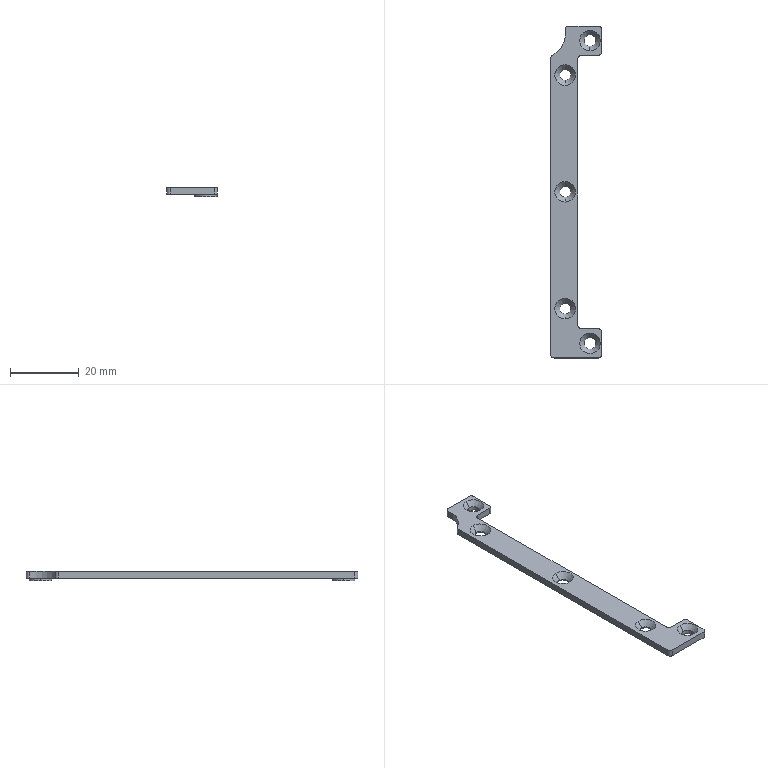Part | 1 solid | 46 faces | box 14.723 x 96.5 x 2.7 mm | volume 1577 mm3 | cylinder 24 | plane 12 | cone 10 | commonest cylinder face diameters 3.2 x6 2 x5 1.6 x4 3.4 x4 6.6 x4 14.8 x1
STEP:
#1=CARTESIAN_POINT('',(7.361,44.,-2.));
#2=VERTEX_POINT('',#1);
#3=CARTESIAN_POINT('',(0.7613,44.,-2.));
#4=VERTEX_POINT('',#3);
#5=CARTESIAN_POINT('',(4.061,44.,-2.));
#6=DIRECTION('',(0.,0.,-1.));
#7=DIRECTION('',(1.,0.,0.));
#8=AXIS2_PLACEMENT_3D('',#5,#6,#7);
#9=CIRCLE('',#8,3.3);
#10=EDGE_CURVE('',#2,#4,#9,.T.);
#11=ORIENTED_EDGE('',*,*,#10,.F.);
#12=CARTESIAN_POINT('',(7.361,40.55,-2.));
#13=VERTEX_POINT('',#12);
#14=CARTESIAN_POINT('',(7.361,40.55,-2.));
#15=DIRECTION('',(0.,1.,0.));
#16=VECTOR('',#15,1000.);
#17=LINE('',#14,#16);
#18=EDGE_CURVE('',#13,#2,#17,.T.);
#19=ORIENTED_EDGE('',*,*,#18,.F.);
#20=CARTESIAN_POINT('',(6.561,39.75,-2.));
#21=VERTEX_POINT('',#20);
#22=CARTESIAN_POINT('',(6.561,40.55,-2.));
#23=DIRECTION('',(0.,0.,1.));
#24=DIRECTION('',(0.,-1.,0.));
#25=AXIS2_PLACEMENT_3D('',#22,#23,#24);
#26=CIRCLE('',#25,0.8);
#27=EDGE_CURVE('',#21,#13,#26,.T.);
#28=ORIENTED_EDGE('',*,*,#27,.F.);
#29=CARTESIAN_POINT('',(1.561,39.75,-2.));
#30=VERTEX_POINT('',#29);
#31=CARTESIAN_POINT('',(1.561,39.75,-2.));
#32=DIRECTION('',(1.,0.,0.));
#33=VECTOR('',#32,1000.);
#34=LINE('',#31,#33);
#35=EDGE_CURVE('',#30,#21,#34,.T.);
#36=ORIENTED_EDGE('',*,*,#35,.F.);
#37=CARTESIAN_POINT('',(0.5613,38.75,-2.));
#38=VERTEX_POINT('',#37);
#39=CARTESIAN_POINT('',(1.561,38.75,-2.));
#40=DIRECTION('',(0.,0.,1.));
#41=DIRECTION('',(0.,1.,0.));
#42=AXIS2_PLACEMENT_3D('',#39,#40,#41);
#43=CIRCLE('',#42,1.);
#44=EDGE_CURVE('',#30,#38,#43,.T.);
#45=ORIENTED_EDGE('',*,*,#44,.T.);
#46=CARTESIAN_POINT('',(0.5613,-38.75,-2.));
#47=VERTEX_POINT('',#46);
#48=CARTESIAN_POINT('',(0.5613,-38.75,-2.));
#49=DIRECTION('',(0.,1.,0.));
#50=VECTOR('',#49,1000.);
#51=LINE('',#48,#50);
#52=EDGE_CURVE('',#47,#38,#51,.T.);
#53=ORIENTED_EDGE('',*,*,#52,.F.);
#54=CARTESIAN_POINT('',(1.561,-39.75,-2.));
#55=VERTEX_POINT('',#54);
#56=CARTESIAN_POINT('',(1.561,-38.75,-2.));
#57=DIRECTION('',(0.,0.,1.));
#58=DIRECTION('',(-1.,0.,0.));
#59=AXIS2_PLACEMENT_3D('',#56,#57,#58);
#60=CIRCLE('',#59,1.);
#61=EDGE_CURVE('',#47,#55,#60,.T.);
#62=ORIENTED_EDGE('',*,*,#61,.T.);
#63=CARTESIAN_POINT('',(6.561,-39.75,-2.));
#64=VERTEX_POINT('',#63);
#65=CARTESIAN_POINT('',(6.561,-39.75,-2.));
#66=DIRECTION('',(-1.,0.,0.));
#67=VECTOR('',#66,1000.);
#68=LINE('',#65,#67);
#69=EDGE_CURVE('',#64,#55,#68,.T.);
#70=ORIENTED_EDGE('',*,*,#69,.F.);
#71=CARTESIAN_POINT('',(7.361,-40.55,-2.));
#72=VERTEX_POINT('',#71);
#73=CARTESIAN_POINT('',(6.561,-40.55,-2.));
#74=DIRECTION('',(0.,0.,1.));
#75=DIRECTION('',(1.,0.,0.));
#76=AXIS2_PLACEMENT_3D('',#73,#74,#75);
#77=CIRCLE('',#76,0.8);
#78=EDGE_CURVE('',#72,#64,#77,.T.);
#79=ORIENTED_EDGE('',*,*,#78,.F.);
#80=CARTESIAN_POINT('',(7.361,-44.,-2.));
#81=VERTEX_POINT('',#80);
#82=CARTESIAN_POINT('',(7.361,-44.,-2.));
#83=DIRECTION('',(0.,1.,0.));
#84=VECTOR('',#83,1000.);
#85=LINE('',#82,#84);
#86=EDGE_CURVE('',#81,#72,#85,.T.);
#87=ORIENTED_EDGE('',*,*,#86,.F.);
#88=CARTESIAN_POINT('',(0.7613,-44.,-2.));
#89=VERTEX_POINT('',#88);
#90=CARTESIAN_POINT('',(4.061,-44.,-2.));
#91=DIRECTION('',(0.,0.,-1.));
#92=DIRECTION('',(-1.,0.,0.));
#93=AXIS2_PLACEMENT_3D('',#90,#91,#92);
#94=CIRCLE('',#93,3.3);
#95=EDGE_CURVE('',#89,#81,#94,.T.);
#96=ORIENTED_EDGE('',*,*,#95,.F.);
#97=CARTESIAN_POINT('',(4.061,-44.,-2.));
#98=DIRECTION('',(0.,0.,-1.));
#99=DIRECTION('',(1.,0.,0.));
#100=AXIS2_PLACEMENT_3D('',#97,#98,#99);
#101=CIRCLE('',#100,3.3);
#102=EDGE_CURVE('',#81,#89,#101,.T.);
#103=ORIENTED_EDGE('',*,*,#102,.F.);
#104=CARTESIAN_POINT('',(7.361,-47.45,-2.));
#105=VERTEX_POINT('',#104);
#106=CARTESIAN_POINT('',(7.361,-47.45,-2.));
#107=DIRECTION('',(0.,1.,0.));
#108=VECTOR('',#107,1000.);
#109=LINE('',#106,#108);
#110=EDGE_CURVE('',#105,#81,#109,.T.);
#111=ORIENTED_EDGE('',*,*,#110,.F.);
#112=CARTESIAN_POINT('',(6.561,-48.25,-2.));
#113=VERTEX_POINT('',#112);
#114=CARTESIAN_POINT('',(6.561,-47.45,-2.));
#115=DIRECTION('',(0.,0.,1.));
#116=DIRECTION('',(0.,-1.,0.));
#117=AXIS2_PLACEMENT_3D('',#114,#115,#116);
#118=CIRCLE('',#117,0.8);
#119=EDGE_CURVE('',#113,#105,#118,.T.);
#120=ORIENTED_EDGE('',*,*,#119,.F.);
#121=CARTESIAN_POINT('',(-6.361,-48.25,-2.));
#122=VERTEX_POINT('',#121);
#123=CARTESIAN_POINT('',(-6.361,-48.25,-2.));
#124=DIRECTION('',(1.,0.,0.));
#125=VECTOR('',#124,1000.);
#126=LINE('',#123,#125);
#127=EDGE_CURVE('',#122,#113,#126,.T.);
#128=ORIENTED_EDGE('',*,*,#127,.F.);
#129=CARTESIAN_POINT('',(-7.361,-47.25,-2.));
#130=VERTEX_POINT('',#129);
#131=CARTESIAN_POINT('',(-6.361,-47.25,-2.));
#132=DIRECTION('',(0.,0.,-1.));
#133=DIRECTION('',(0.,-1.,0.));
#134=AXIS2_PLACEMENT_3D('',#131,#132,#133);
#135=CIRCLE('',#134,1.);
#136=EDGE_CURVE('',#122,#130,#135,.T.);
#137=ORIENTED_EDGE('',*,*,#136,.T.);
#138=CARTESIAN_POINT('',(-7.361,38.806,-2.));
#139=VERTEX_POINT('',#138);
#140=CARTESIAN_POINT('',(-7.361,38.806,-2.));
#141=DIRECTION('',(0.,-1.,0.));
#142=VECTOR('',#141,1000.);
#143=LINE('',#140,#142);
#144=EDGE_CURVE('',#139,#130,#143,.T.);
#145=ORIENTED_EDGE('',*,*,#144,.F.);
#146=CARTESIAN_POINT('',(-6.847,39.68,-2.));
#147=VERTEX_POINT('',#146);
#148=CARTESIAN_POINT('',(-6.361,38.806,-2.));
#149=DIRECTION('',(0.,0.,-1.));
#150=DIRECTION('',(-1.,0.,0.));
#151=AXIS2_PLACEMENT_3D('',#148,#149,#150);
#152=CIRCLE('',#151,1.);
#153=EDGE_CURVE('',#139,#147,#152,.T.);
#154=ORIENTED_EDGE('',*,*,#153,.T.);
#155=CARTESIAN_POINT('',(-3.102,47.119,-2.));
#156=VERTEX_POINT('',#155);
#157=CARTESIAN_POINT('',(-10.439,46.15,-2.));
#158=DIRECTION('',(0.,0.,-1.));
#159=DIRECTION('',(0.9914,0.131,0.));
#160=AXIS2_PLACEMENT_3D('',#157,#158,#159);
#161=CIRCLE('',#160,7.4);
#162=EDGE_CURVE('',#156,#147,#161,.T.);
#163=ORIENTED_EDGE('',*,*,#162,.F.);
#164=CARTESIAN_POINT('',(-2.111,48.25,-2.));
#165=VERTEX_POINT('',#164);
#166=CARTESIAN_POINT('',(-2.111,47.25,-2.));
#167=DIRECTION('',(0.,0.,-1.));
#168=DIRECTION('',(-0.9914,-0.131,0.));
#169=AXIS2_PLACEMENT_3D('',#166,#167,#168);
#170=CIRCLE('',#169,1.);
#171=EDGE_CURVE('',#156,#165,#170,.T.);
#172=ORIENTED_EDGE('',*,*,#171,.T.);
#173=CARTESIAN_POINT('',(6.561,48.25,-2.));
#174=VERTEX_POINT('',#173);
#175=CARTESIAN_POINT('',(6.561,48.25,-2.));
#176=DIRECTION('',(-1.,0.,0.));
#177=VECTOR('',#176,1000.);
#178=LINE('',#175,#177);
#179=EDGE_CURVE('',#174,#165,#178,.T.);
#180=ORIENTED_EDGE('',*,*,#179,.F.);
#181=CARTESIAN_POINT('',(7.361,47.45,-2.));
#182=VERTEX_POINT('',#181);
#183=CARTESIAN_POINT('',(6.561,47.45,-2.));
#184=DIRECTION('',(0.,0.,1.));
#185=DIRECTION('',(1.,0.,0.));
#186=AXIS2_PLACEMENT_3D('',#183,#184,#185);
#187=CIRCLE('',#186,0.8);
#188=EDGE_CURVE('',#182,#174,#187,.T.);
#189=ORIENTED_EDGE('',*,*,#188,.F.);
#190=CARTESIAN_POINT('',(7.361,44.,-2.));
#191=DIRECTION('',(0.,1.,0.));
#192=VECTOR('',#191,1000.);
#193=LINE('',#190,#192);
#194=EDGE_CURVE('',#2,#182,#193,.T.);
#195=ORIENTED_EDGE('',*,*,#194,.F.);
#196=CARTESIAN_POINT('',(4.061,44.,-2.));
#197=DIRECTION('',(0.,0.,-1.));
#198=DIRECTION('',(-1.,0.,0.));
#199=AXIS2_PLACEMENT_3D('',#196,#197,#198);
#200=CIRCLE('',#199,3.3);
#201=EDGE_CURVE('',#4,#2,#200,.T.);
#202=ORIENTED_EDGE('',*,*,#201,.F.);
#203=EDGE_LOOP('',(#11,#19,#28,#36,#45,#53,#62,#70,#79,#87,#96,#103,#111,#120,#128,#137,#145,#154,#163,#172,#180,#189,#195,#202));
#204=FACE_BOUND('',#203,.T.);
#205=CARTESIAN_POINT('',(-4.75,0.05,-2.));
#206=VERTEX_POINT('',#205);
#207=CARTESIAN_POINT('',(-1.55,0.05,-2.));
#208=VERTEX_POINT('',#207);
#209=CARTESIAN_POINT('',(-3.15,0.05,-2.));
#210=DIRECTION('',(0.,0.,1.));
#211=DIRECTION('',(-1.,0.,0.));
#212=AXIS2_PLACEMENT_3D('',#209,#210,#211);
#213=CIRCLE('',#212,1.6);
#214=EDGE_CURVE('',#206,#208,#213,.T.);
#215=ORIENTED_EDGE('',*,*,#214,.T.);
#216=CARTESIAN_POINT('',(-3.15,0.05,-2.));
#217=DIRECTION('',(0.,0.,1.));
#218=DIRECTION('',(1.,0.,0.));
#219=AXIS2_PLACEMENT_3D('',#216,#217,#218);
#220=CIRCLE('',#219,1.6);
#221=EDGE_CURVE('',#208,#206,#220,.T.);
#222=ORIENTED_EDGE('',*,*,#221,.T.);
#223=EDGE_LOOP('',(#215,#222));
#224=FACE_BOUND('',#223,.T.);
#225=CARTESIAN_POINT('',(-4.75,-33.9,-2.));
#226=VERTEX_POINT('',#225);
#227=CARTESIAN_POINT('',(-1.55,-33.9,-2.));
#228=VERTEX_POINT('',#227);
#229=CARTESIAN_POINT('',(-3.15,-33.9,-2.));
#230=DIRECTION('',(0.,0.,1.));
#231=DIRECTION('',(-1.,0.,0.));
#232=AXIS2_PLACEMENT_3D('',#229,#230,#231);
#233=CIRCLE('',#232,1.6);
#234=EDGE_CURVE('',#226,#228,#233,.T.);
#235=ORIENTED_EDGE('',*,*,#234,.T.);
#236=CARTESIAN_POINT('',(-3.15,-33.9,-2.));
#237=DIRECTION('',(0.,0.,1.));
#238=DIRECTION('',(1.,0.,0.));
#239=AXIS2_PLACEMENT_3D('',#236,#237,#238);
#240=CIRCLE('',#239,1.6);
#241=EDGE_CURVE('',#228,#226,#240,.T.);
#242=ORIENTED_EDGE('',*,*,#241,.T.);
#243=EDGE_LOOP('',(#235,#242));
#244=FACE_BOUND('',#243,.T.);
#245=CARTESIAN_POINT('',(-4.75,34.,-2.));
#246=VERTEX_POINT('',#245);
#247=CARTESIAN_POINT('',(-1.55,34.,-2.));
#248=VERTEX_POINT('',#247);
#249=CARTESIAN_POINT('',(-3.15,34.,-2.));
#250=DIRECTION('',(0.,0.,1.));
#251=DIRECTION('',(-1.,0.,0.));
#252=AXIS2_PLACEMENT_3D('',#249,#250,#251);
#253=CIRCLE('',#252,1.6);
#254=EDGE_CURVE('',#246,#248,#253,.T.);
#255=ORIENTED_EDGE('',*,*,#254,.T.);
#256=CARTESIAN_POINT('',(-3.15,34.,-2.));
#257=DIRECTION('',(0.,0.,1.));
#258=DIRECTION('',(1.,0.,0.));
#259=AXIS2_PLACEMENT_3D('',#256,#257,#258);
#260=CIRCLE('',#259,1.6);
#261=EDGE_CURVE('',#248,#246,#260,.T.);
#262=ORIENTED_EDGE('',*,*,#261,.T.);
#263=EDGE_LOOP('',(#255,#262));
#264=FACE_BOUND('',#263,.T.);
#265=CARTESIAN_POINT('',(100.961,0.05,-2.));
#266=DIRECTION('',(0.,0.,1.));
#267=DIRECTION('',(-1.,0.,0.));
#268=AXIS2_PLACEMENT_3D('',#265,#266,#267);
#269=PLANE('',#268);
#270=ADVANCED_FACE('',(#204,#224,#244,#264),#269,.F.);
#271=CARTESIAN_POINT('',(-4.75,34.,-1.68));
#272=VERTEX_POINT('',#271);
#273=CARTESIAN_POINT('',(-4.75,34.,-2.));
#274=DIRECTION('',(0.,0.,1.));
#275=VECTOR('',#274,1000.);
#276=LINE('',#273,#275);
#277=EDGE_CURVE('',#272,#246,#276,.F.);
#278=ORIENTED_EDGE('',*,*,#277,.T.);
#279=ORIENTED_EDGE('',*,*,#261,.F.);
#280=CARTESIAN_POINT('',(-1.55,34.,-1.68));
#281=VERTEX_POINT('',#280);
#282=CARTESIAN_POINT('',(-1.55,34.,-2.));
#283=DIRECTION('',(0.,0.,1.));
#284=VECTOR('',#283,1000.);
#285=LINE('',#282,#284);
#286=EDGE_CURVE('',#281,#248,#285,.F.);
#287=ORIENTED_EDGE('',*,*,#286,.F.);
#288=CARTESIAN_POINT('',(-3.15,35.6,-1.68));
#289=VERTEX_POINT('',#288);
#290=CARTESIAN_POINT('',(-3.15,34.,-1.68));
#291=DIRECTION('',(0.,0.,1.));
#292=DIRECTION('',(1.,0.,0.));
#293=AXIS2_PLACEMENT_3D('',#290,#291,#292);
#294=CIRCLE('',#293,1.6);
#295=EDGE_CURVE('',#281,#289,#294,.T.);
#296=ORIENTED_EDGE('',*,*,#295,.T.);
#297=CARTESIAN_POINT('',(-3.15,34.,-1.68));
#298=DIRECTION('',(0.,0.,1.));
#299=DIRECTION('',(0.,1.,0.));
#300=AXIS2_PLACEMENT_3D('',#297,#298,#299);
#301=CIRCLE('',#300,1.6);
#302=EDGE_CURVE('',#289,#272,#301,.T.);
#303=ORIENTED_EDGE('',*,*,#302,.T.);
#304=EDGE_LOOP('',(#278,#279,#287,#296,#303));
#305=FACE_BOUND('',#304,.T.);
#306=CARTESIAN_POINT('',(-3.15,34.,-44.195));
#307=DIRECTION('',(0.,0.,1.));
#308=DIRECTION('',(-1.,0.,0.));
#309=AXIS2_PLACEMENT_3D('',#306,#307,#308);
#310=CYLINDRICAL_SURFACE('',#309,1.6);
#311=ADVANCED_FACE('',(#305),#310,.F.);
#312=CARTESIAN_POINT('',(-3.15,32.4,-1.68));
#313=VERTEX_POINT('',#312);
#314=CARTESIAN_POINT('',(-3.15,31.,0.));
#315=VERTEX_POINT('',#314);
#316=CARTESIAN_POINT('',(-3.15,32.4,-1.68));
#317=DIRECTION('',(0.,-0.6402,0.7682));
#318=VECTOR('',#317,1000.);
#319=LINE('',#316,#318);
#320=EDGE_CURVE('',#313,#315,#319,.T.);
#321=ORIENTED_EDGE('',*,*,#320,.F.);
#322=CARTESIAN_POINT('',(-3.15,34.,-1.68));
#323=DIRECTION('',(0.,0.,1.));
#324=DIRECTION('',(-1.,0.,0.));
#325=AXIS2_PLACEMENT_3D('',#322,#323,#324);
#326=CIRCLE('',#325,1.6);
#327=EDGE_CURVE('',#272,#313,#326,.T.);
#328=ORIENTED_EDGE('',*,*,#327,.F.);
#329=ORIENTED_EDGE('',*,*,#302,.F.);
#330=CARTESIAN_POINT('',(-3.15,37.,0.));
#331=VERTEX_POINT('',#330);
#332=CARTESIAN_POINT('',(-3.15,35.6,-1.68));
#333=DIRECTION('',(0.,0.6402,0.7682));
#334=VECTOR('',#333,1000.);
#335=LINE('',#332,#334);
#336=EDGE_CURVE('',#289,#331,#335,.T.);
#337=ORIENTED_EDGE('',*,*,#336,.T.);
#338=CARTESIAN_POINT('',(-3.15,34.,0.));
#339=DIRECTION('',(0.,0.,-1.));
#340=DIRECTION('',(0.,-1.,0.));
#341=AXIS2_PLACEMENT_3D('',#338,#339,#340);
#342=CIRCLE('',#341,3.);
#343=EDGE_CURVE('',#315,#331,#342,.T.);
#344=ORIENTED_EDGE('',*,*,#343,.F.);
#345=EDGE_LOOP('',(#321,#328,#329,#337,#344));
#346=FACE_BOUND('',#345,.T.);
#347=CARTESIAN_POINT('',(-3.15,34.,-0.84));
#348=DIRECTION('',(0.,0.,1.));
#349=DIRECTION('',(0.,1.,0.));
#350=AXIS2_PLACEMENT_3D('',#347,#348,#349);
#351=CONICAL_SURFACE('',#350,2.3,0.6947);
#352=ADVANCED_FACE('',(#346),#351,.F.);
#353=CARTESIAN_POINT('',(-3.102,47.119,0.));
#354=VERTEX_POINT('',#353);
#355=CARTESIAN_POINT('',(-6.847,39.68,0.));
#356=VERTEX_POINT('',#355);
#357=CARTESIAN_POINT('',(-10.439,46.15,0.));
#358=DIRECTION('',(0.,0.,-1.));
#359=DIRECTION('',(0.9914,0.131,0.));
#360=AXIS2_PLACEMENT_3D('',#357,#358,#359);
#361=CIRCLE('',#360,7.4);
#362=EDGE_CURVE('',#354,#356,#361,.T.);
#363=ORIENTED_EDGE('',*,*,#362,.T.);
#364=CARTESIAN_POINT('',(-7.361,38.806,0.));
#365=VERTEX_POINT('',#364);
#366=CARTESIAN_POINT('',(-6.361,38.806,0.));
#367=DIRECTION('',(0.,0.,1.));
#368=DIRECTION('',(-0.4854,0.8743,0.));
#369=AXIS2_PLACEMENT_3D('',#366,#367,#368);
#370=CIRCLE('',#369,1.);
#371=EDGE_CURVE('',#356,#365,#370,.T.);
#372=ORIENTED_EDGE('',*,*,#371,.T.);
#373=CARTESIAN_POINT('',(-7.361,-47.25,0.));
#374=VERTEX_POINT('',#373);
#375=CARTESIAN_POINT('',(-7.361,38.806,0.));
#376=DIRECTION('',(0.,-1.,0.));
#377=VECTOR('',#376,1000.);
#378=LINE('',#375,#377);
#379=EDGE_CURVE('',#365,#374,#378,.T.);
#380=ORIENTED_EDGE('',*,*,#379,.T.);
#381=CARTESIAN_POINT('',(-6.361,-48.25,0.));
#382=VERTEX_POINT('',#381);
#383=CARTESIAN_POINT('',(-6.361,-47.25,0.));
#384=DIRECTION('',(0.,0.,1.));
#385=DIRECTION('',(-1.,0.,0.));
#386=AXIS2_PLACEMENT_3D('',#383,#384,#385);
#387=CIRCLE('',#386,1.);
#388=EDGE_CURVE('',#374,#382,#387,.T.);
#389=ORIENTED_EDGE('',*,*,#388,.T.);
#390=CARTESIAN_POINT('',(6.561,-48.25,0.));
#391=VERTEX_POINT('',#390);
#392=CARTESIAN_POINT('',(-6.361,-48.25,0.));
#393=DIRECTION('',(1.,0.,0.));
#394=VECTOR('',#393,1000.);
#395=LINE('',#392,#394);
#396=EDGE_CURVE('',#382,#391,#395,.T.);
#397=ORIENTED_EDGE('',*,*,#396,.T.);
#398=CARTESIAN_POINT('',(7.361,-47.45,0.));
#399=VERTEX_POINT('',#398);
#400=CARTESIAN_POINT('',(6.561,-47.45,0.));
#401=DIRECTION('',(0.,0.,1.));
#402=DIRECTION('',(0.,-1.,0.));
#403=AXIS2_PLACEMENT_3D('',#400,#401,#402);
#404=CIRCLE('',#403,0.8);
#405=EDGE_CURVE('',#391,#399,#404,.T.);
#406=ORIENTED_EDGE('',*,*,#405,.T.);
#407=CARTESIAN_POINT('',(7.361,-40.55,0.));
#408=VERTEX_POINT('',#407);
#409=CARTESIAN_POINT('',(7.361,-47.45,0.));
#410=DIRECTION('',(0.,1.,0.));
#411=VECTOR('',#410,1000.);
#412=LINE('',#409,#411);
#413=EDGE_CURVE('',#399,#408,#412,.T.);
#414=ORIENTED_EDGE('',*,*,#413,.T.);
#415=CARTESIAN_POINT('',(6.561,-39.75,0.));
#416=VERTEX_POINT('',#415);
#417=CARTESIAN_POINT('',(6.561,-40.55,0.));
#418=DIRECTION('',(0.,0.,1.));
#419=DIRECTION('',(1.,0.,0.));
#420=AXIS2_PLACEMENT_3D('',#417,#418,#419);
#421=CIRCLE('',#420,0.8);
#422=EDGE_CURVE('',#408,#416,#421,.T.);
#423=ORIENTED_EDGE('',*,*,#422,.T.);
#424=CARTESIAN_POINT('',(1.561,-39.75,0.));
#425=VERTEX_POINT('',#424);
#426=CARTESIAN_POINT('',(6.561,-39.75,0.));
#427=DIRECTION('',(-1.,0.,0.));
#428=VECTOR('',#427,1000.);
#429=LINE('',#426,#428);
#430=EDGE_CURVE('',#416,#425,#429,.T.);
#431=ORIENTED_EDGE('',*,*,#430,.T.);
#432=CARTESIAN_POINT('',(0.5613,-38.75,0.));
#433=VERTEX_POINT('',#432);
#434=CARTESIAN_POINT('',(1.561,-38.75,0.));
#435=DIRECTION('',(0.,0.,-1.));
#436=DIRECTION('',(0.,-1.,0.));
#437=AXIS2_PLACEMENT_3D('',#434,#435,#436);
#438=CIRCLE('',#437,1.);
#439=EDGE_CURVE('',#425,#433,#438,.T.);
#440=ORIENTED_EDGE('',*,*,#439,.T.);
#441=CARTESIAN_POINT('',(0.5613,38.75,0.));
#442=VERTEX_POINT('',#441);
#443=CARTESIAN_POINT('',(0.5613,-38.75,0.));
#444=DIRECTION('',(0.,1.,0.));
#445=VECTOR('',#444,1000.);
#446=LINE('',#443,#445);
#447=EDGE_CURVE('',#433,#442,#446,.T.);
#448=ORIENTED_EDGE('',*,*,#447,.T.);
#449=CARTESIAN_POINT('',(1.561,39.75,0.));
#450=VERTEX_POINT('',#449);
#451=CARTESIAN_POINT('',(1.561,38.75,0.));
#452=DIRECTION('',(0.,0.,-1.));
#453=DIRECTION('',(-1.,0.,0.));
#454=AXIS2_PLACEMENT_3D('',#451,#452,#453);
#455=CIRCLE('',#454,1.);
#456=EDGE_CURVE('',#442,#450,#455,.T.);
#457=ORIENTED_EDGE('',*,*,#456,.T.);
#458=CARTESIAN_POINT('',(6.561,39.75,0.));
#459=VERTEX_POINT('',#458);
#460=CARTESIAN_POINT('',(1.561,39.75,0.));
#461=DIRECTION('',(1.,0.,0.));
#462=VECTOR('',#461,1000.);
#463=LINE('',#460,#462);
#464=EDGE_CURVE('',#450,#459,#463,.T.);
#465=ORIENTED_EDGE('',*,*,#464,.T.);
#466=CARTESIAN_POINT('',(7.361,40.55,0.));
#467=VERTEX_POINT('',#466);
#468=CARTESIAN_POINT('',(6.561,40.55,0.));
#469=DIRECTION('',(0.,0.,1.));
#470=DIRECTION('',(0.,-1.,0.));
#471=AXIS2_PLACEMENT_3D('',#468,#469,#470);
#472=CIRCLE('',#471,0.8);
#473=EDGE_CURVE('',#459,#467,#472,.T.);
#474=ORIENTED_EDGE('',*,*,#473,.T.);
#475=CARTESIAN_POINT('',(7.361,47.45,0.));
#476=VERTEX_POINT('',#475);
#477=CARTESIAN_POINT('',(7.361,40.55,0.));
#478=DIRECTION('',(0.,1.,0.));
#479=VECTOR('',#478,1000.);
#480=LINE('',#477,#479);
#481=EDGE_CURVE('',#467,#476,#480,.T.);
#482=ORIENTED_EDGE('',*,*,#481,.T.);
#483=CARTESIAN_POINT('',(6.561,48.25,0.));
#484=VERTEX_POINT('',#483);
#485=CARTESIAN_POINT('',(6.561,47.45,0.));
#486=DIRECTION('',(0.,0.,1.));
#487=DIRECTION('',(1.,0.,0.));
#488=AXIS2_PLACEMENT_3D('',#485,#486,#487);
#489=CIRCLE('',#488,0.8);
#490=EDGE_CURVE('',#476,#484,#489,.T.);
#491=ORIENTED_EDGE('',*,*,#490,.T.);
#492=CARTESIAN_POINT('',(-2.111,48.25,0.));
#493=VERTEX_POINT('',#492);
#494=CARTESIAN_POINT('',(6.561,48.25,0.));
#495=DIRECTION('',(-1.,0.,0.));
#496=VECTOR('',#495,1000.);
#497=LINE('',#494,#496);
#498=EDGE_CURVE('',#484,#493,#497,.T.);
#499=ORIENTED_EDGE('',*,*,#498,.T.);
#500=CARTESIAN_POINT('',(-2.111,47.25,0.));
#501=DIRECTION('',(0.,0.,1.));
#502=DIRECTION('',(0.,1.,0.));
#503=AXIS2_PLACEMENT_3D('',#500,#501,#502);
#504=CIRCLE('',#503,1.);
#505=EDGE_CURVE('',#493,#354,#504,.T.);
#506=ORIENTED_EDGE('',*,*,#505,.T.);
#507=EDGE_LOOP('',(#363,#372,#380,#389,#397,#406,#414,#423,#431,#440,#448,#457,#465,#474,#482,#491,#499,#506));
#508=FACE_BOUND('',#507,.T.);
#509=CARTESIAN_POINT('',(4.061,47.,0.));
#510=VERTEX_POINT('',#509);
#511=CARTESIAN_POINT('',(4.061,41.,0.));
#512=VERTEX_POINT('',#511);
#513=CARTESIAN_POINT('',(4.061,44.,0.));
#514=DIRECTION('',(0.,0.,-1.));
#515=DIRECTION('',(0.,1.,0.));
#516=AXIS2_PLACEMENT_3D('',#513,#514,#515);
#517=CIRCLE('',#516,3.);
#518=EDGE_CURVE('',#510,#512,#517,.T.);
#519=ORIENTED_EDGE('',*,*,#518,.T.);
#520=CARTESIAN_POINT('',(4.061,44.,0.));
#521=DIRECTION('',(0.,0.,-1.));
#522=DIRECTION('',(0.,-1.,0.));
#523=AXIS2_PLACEMENT_3D('',#520,#521,#522);
#524=CIRCLE('',#523,3.);
#525=EDGE_CURVE('',#512,#510,#524,.T.);
#526=ORIENTED_EDGE('',*,*,#525,.T.);
#527=EDGE_LOOP('',(#519,#526));
#528=FACE_BOUND('',#527,.T.);
#529=CARTESIAN_POINT('',(-3.15,34.,0.));
#530=DIRECTION('',(0.,0.,-1.));
#531=DIRECTION('',(0.,1.,0.));
#532=AXIS2_PLACEMENT_3D('',#529,#530,#531);
#533=CIRCLE('',#532,3.);
#534=EDGE_CURVE('',#331,#315,#533,.T.);
#535=ORIENTED_EDGE('',*,*,#534,.T.);
#536=ORIENTED_EDGE('',*,*,#343,.T.);
#537=EDGE_LOOP('',(#535,#536));
#538=FACE_BOUND('',#537,.T.);
#539=CARTESIAN_POINT('',(-3.15,3.05,0.));
#540=VERTEX_POINT('',#539);
#541=CARTESIAN_POINT('',(-3.15,-2.95,0.));
#542=VERTEX_POINT('',#541);
#543=CARTESIAN_POINT('',(-3.15,0.05,0.));
#544=DIRECTION('',(0.,0.,-1.));
#545=DIRECTION('',(0.,1.,0.));
#546=AXIS2_PLACEMENT_3D('',#543,#544,#545);
#547=CIRCLE('',#546,3.);
#548=EDGE_CURVE('',#540,#542,#547,.T.);
#549=ORIENTED_EDGE('',*,*,#548,.T.);
#550=CARTESIAN_POINT('',(-3.15,0.05,0.));
#551=DIRECTION('',(0.,0.,-1.));
#552=DIRECTION('',(0.,-1.,0.));
#553=AXIS2_PLACEMENT_3D('',#550,#551,#552);
#554=CIRCLE('',#553,3.);
#555=EDGE_CURVE('',#542,#540,#554,.T.);
#556=ORIENTED_EDGE('',*,*,#555,.T.);
#557=EDGE_LOOP('',(#549,#556));
#558=FACE_BOUND('',#557,.T.);
#559=CARTESIAN_POINT('',(-3.15,-30.9,0.));
#560=VERTEX_POINT('',#559);
#561=CARTESIAN_POINT('',(-3.15,-36.9,0.));
#562=VERTEX_POINT('',#561);
#563=CARTESIAN_POINT('',(-3.15,-33.9,0.));
#564=DIRECTION('',(0.,0.,-1.));
#565=DIRECTION('',(0.,1.,0.));
#566=AXIS2_PLACEMENT_3D('',#563,#564,#565);
#567=CIRCLE('',#566,3.);
#568=EDGE_CURVE('',#560,#562,#567,.T.);
#569=ORIENTED_EDGE('',*,*,#568,.T.);
#570=CARTESIAN_POINT('',(-3.15,-33.9,0.));
#571=DIRECTION('',(0.,0.,-1.));
#572=DIRECTION('',(0.,-1.,0.));
#573=AXIS2_PLACEMENT_3D('',#570,#571,#572);
#574=CIRCLE('',#573,3.);
#575=EDGE_CURVE('',#562,#560,#574,.T.);
#576=ORIENTED_EDGE('',*,*,#575,.T.);
#577=EDGE_LOOP('',(#569,#576));
#578=FACE_BOUND('',#577,.T.);
#579=CARTESIAN_POINT('',(4.061,-41.,0.));
#580=VERTEX_POINT('',#579);
#581=CARTESIAN_POINT('',(4.061,-47.,0.));
#582=VERTEX_POINT('',#581);
#583=CARTESIAN_POINT('',(4.061,-44.,0.));
#584=DIRECTION('',(0.,0.,-1.));
#585=DIRECTION('',(0.,1.,0.));
#586=AXIS2_PLACEMENT_3D('',#583,#584,#585);
#587=CIRCLE('',#586,3.);
#588=EDGE_CURVE('',#580,#582,#587,.T.);
#589=ORIENTED_EDGE('',*,*,#588,.T.);
#590=CARTESIAN_POINT('',(4.061,-44.,0.));
#591=DIRECTION('',(0.,0.,-1.));
#592=DIRECTION('',(0.,-1.,0.));
#593=AXIS2_PLACEMENT_3D('',#590,#591,#592);
#594=CIRCLE('',#593,3.);
#595=EDGE_CURVE('',#582,#580,#594,.T.);
#596=ORIENTED_EDGE('',*,*,#595,.T.);
#597=EDGE_LOOP('',(#589,#596));
#598=FACE_BOUND('',#597,.T.);
#599=CARTESIAN_POINT('',(100.961,0.05,0.));
#600=DIRECTION('',(0.,0.,1.));
#601=DIRECTION('',(-1.,0.,0.));
#602=AXIS2_PLACEMENT_3D('',#599,#600,#601);
#603=PLANE('',#602);
#604=ADVANCED_FACE('',(#508,#528,#538,#558,#578,#598),#603,.T.);
#605=CARTESIAN_POINT('',(-3.102,47.119,0.));
#606=DIRECTION('',(0.,0.,-1.));
#607=VECTOR('',#606,1000.);
#608=LINE('',#605,#607);
#609=EDGE_CURVE('',#354,#156,#608,.T.);
#610=ORIENTED_EDGE('',*,*,#609,.F.);
#611=ORIENTED_EDGE('',*,*,#505,.F.);
#612=CARTESIAN_POINT('',(-2.111,48.25,0.));
#613=DIRECTION('',(0.,0.,-1.));
#614=VECTOR('',#613,1000.);
#615=LINE('',#612,#614);
#616=EDGE_CURVE('',#493,#165,#615,.T.);
#617=ORIENTED_EDGE('',*,*,#616,.T.);
#618=ORIENTED_EDGE('',*,*,#171,.F.);
#619=EDGE_LOOP('',(#610,#611,#617,#618));
#620=FACE_BOUND('',#619,.T.);
#621=CARTESIAN_POINT('',(-2.111,47.25,153.925));
#622=DIRECTION('',(0.,0.,-1.));
#623=DIRECTION('',(0.9914,0.131,0.));
#624=AXIS2_PLACEMENT_3D('',#621,#622,#623);
#625=CYLINDRICAL_SURFACE('',#624,1.);
#626=ADVANCED_FACE('',(#620),#625,.T.);
#627=ORIENTED_EDGE('',*,*,#498,.F.);
#628=CARTESIAN_POINT('',(6.561,48.25,-2.));
#629=DIRECTION('',(0.,0.,1.));
#630=VECTOR('',#629,1000.);
#631=LINE('',#628,#630);
#632=EDGE_CURVE('',#174,#484,#631,.T.);
#633=ORIENTED_EDGE('',*,*,#632,.F.);
#634=ORIENTED_EDGE('',*,*,#179,.T.);
#635=ORIENTED_EDGE('',*,*,#616,.F.);
#636=EDGE_LOOP('',(#627,#633,#634,#635));
#637=FACE_BOUND('',#636,.T.);
#638=CARTESIAN_POINT('',(6.561,48.25,-2.));
#639=DIRECTION('',(0.,1.,0.));
#640=DIRECTION('',(1.,0.,0.));
#641=AXIS2_PLACEMENT_3D('',#638,#639,#640);
#642=PLANE('',#641);
#643=ADVANCED_FACE('',(#637),#642,.T.);
#644=ORIENTED_EDGE('',*,*,#632,.T.);
#645=ORIENTED_EDGE('',*,*,#490,.F.);
#646=CARTESIAN_POINT('',(7.361,47.45,-2.));
#647=DIRECTION('',(0.,0.,1.));
#648=VECTOR('',#647,1000.);
#649=LINE('',#646,#648);
#650=EDGE_CURVE('',#182,#476,#649,.T.);
#651=ORIENTED_EDGE('',*,*,#650,.F.);
#652=ORIENTED_EDGE('',*,*,#188,.T.);
#653=EDGE_LOOP('',(#644,#645,#651,#652));
#654=FACE_BOUND('',#653,.T.);
#655=CARTESIAN_POINT('',(6.561,47.45,-2.));
#656=DIRECTION('',(0.,0.,1.));
#657=DIRECTION('',(-1.,0.,0.));
#658=AXIS2_PLACEMENT_3D('',#655,#656,#657);
#659=CYLINDRICAL_SURFACE('',#658,0.8);
#660=ADVANCED_FACE('',(#654),#659,.T.);
#661=ORIENTED_EDGE('',*,*,#194,.T.);
#662=ORIENTED_EDGE('',*,*,#650,.T.);
#663=ORIENTED_EDGE('',*,*,#481,.F.);
#664=CARTESIAN_POINT('',(7.361,40.55,-2.));
#665=DIRECTION('',(0.,0.,1.));
#666=VECTOR('',#665,1000.);
#667=LINE('',#664,#666);
#668=EDGE_CURVE('',#13,#467,#667,.T.);
#669=ORIENTED_EDGE('',*,*,#668,.F.);
#670=ORIENTED_EDGE('',*,*,#18,.T.);
#671=EDGE_LOOP('',(#661,#662,#663,#669,#670));
#672=FACE_BOUND('',#671,.T.);
#673=CARTESIAN_POINT('',(7.361,40.55,-2.));
#674=DIRECTION('',(1.,0.,0.));
#675=DIRECTION('',(0.,-1.,0.));
#676=AXIS2_PLACEMENT_3D('',#673,#674,#675);
#677=PLANE('',#676);
#678=ADVANCED_FACE('',(#672),#677,.T.);
#679=ORIENTED_EDGE('',*,*,#668,.T.);
#680=ORIENTED_EDGE('',*,*,#473,.F.);
#681=CARTESIAN_POINT('',(6.561,39.75,-2.));
#682=DIRECTION('',(0.,0.,1.));
#683=VECTOR('',#682,1000.);
#684=LINE('',#681,#683);
#685=EDGE_CURVE('',#21,#459,#684,.T.);
#686=ORIENTED_EDGE('',*,*,#685,.F.);
#687=ORIENTED_EDGE('',*,*,#27,.T.);
#688=EDGE_LOOP('',(#679,#680,#686,#687));
#689=FACE_BOUND('',#688,.T.);
#690=CARTESIAN_POINT('',(6.561,40.55,-2.));
#691=DIRECTION('',(0.,0.,1.));
#692=DIRECTION('',(-1.,0.,0.));
#693=AXIS2_PLACEMENT_3D('',#690,#691,#692);
#694=CYLINDRICAL_SURFACE('',#693,0.8);
#695=ADVANCED_FACE('',(#689),#694,.T.);
#696=ORIENTED_EDGE('',*,*,#35,.T.);
#697=ORIENTED_EDGE('',*,*,#685,.T.);
#698=ORIENTED_EDGE('',*,*,#464,.F.);
#699=CARTESIAN_POINT('',(1.561,39.75,-2.));
#700=DIRECTION('',(0.,0.,1.));
#701=VECTOR('',#700,1000.);
#702=LINE('',#699,#701);
#703=EDGE_CURVE('',#30,#450,#702,.T.);
#704=ORIENTED_EDGE('',*,*,#703,.F.);
#705=EDGE_LOOP('',(#696,#697,#698,#704));
#706=FACE_BOUND('',#705,.T.);
#707=CARTESIAN_POINT('',(1.261,39.75,-2.));
#708=DIRECTION('',(0.,-1.,0.));
#709=DIRECTION('',(-1.,0.,0.));
#710=AXIS2_PLACEMENT_3D('',#707,#708,#709);
#711=PLANE('',#710);
#712=ADVANCED_FACE('',(#706),#711,.T.);
#713=ORIENTED_EDGE('',*,*,#456,.F.);
#714=CARTESIAN_POINT('',(0.5613,38.75,-2.));
#715=DIRECTION('',(0.,0.,1.));
#716=VECTOR('',#715,1000.);
#717=LINE('',#714,#716);
#718=EDGE_CURVE('',#38,#442,#717,.T.);
#719=ORIENTED_EDGE('',*,*,#718,.F.);
#720=ORIENTED_EDGE('',*,*,#44,.F.);
#721=ORIENTED_EDGE('',*,*,#703,.T.);
#722=EDGE_LOOP('',(#713,#719,#720,#721));
#723=FACE_BOUND('',#722,.T.);
#724=CARTESIAN_POINT('',(1.561,38.75,-113.446));
#725=DIRECTION('',(0.,0.,1.));
#726=DIRECTION('',(0.,-1.,0.));
#727=AXIS2_PLACEMENT_3D('',#724,#725,#726);
#728=CYLINDRICAL_SURFACE('',#727,1.);
#729=ADVANCED_FACE('',(#723),#728,.F.);
#730=ORIENTED_EDGE('',*,*,#52,.T.);
#731=ORIENTED_EDGE('',*,*,#718,.T.);
#732=ORIENTED_EDGE('',*,*,#447,.F.);
#733=CARTESIAN_POINT('',(0.5613,-38.75,-2.));
#734=DIRECTION('',(0.,0.,1.));
#735=VECTOR('',#734,1000.);
#736=LINE('',#733,#735);
#737=EDGE_CURVE('',#47,#433,#736,.T.);
#738=ORIENTED_EDGE('',*,*,#737,.F.);
#739=EDGE_LOOP('',(#730,#731,#732,#738));
#740=FACE_BOUND('',#739,.T.);
#741=CARTESIAN_POINT('',(0.5613,-39.55,-2.));
#742=DIRECTION('',(1.,0.,0.));
#743=DIRECTION('',(0.,-1.,0.));
#744=AXIS2_PLACEMENT_3D('',#741,#742,#743);
#745=PLANE('',#744);
#746=ADVANCED_FACE('',(#740),#745,.T.);
#747=ORIENTED_EDGE('',*,*,#439,.F.);
#748=CARTESIAN_POINT('',(1.561,-39.75,-2.));
#749=DIRECTION('',(0.,0.,1.));
#750=VECTOR('',#749,1000.);
#751=LINE('',#748,#750);
#752=EDGE_CURVE('',#55,#425,#751,.T.);
#753=ORIENTED_EDGE('',*,*,#752,.F.);
#754=ORIENTED_EDGE('',*,*,#61,.F.);
#755=ORIENTED_EDGE('',*,*,#737,.T.);
#756=EDGE_LOOP('',(#747,#753,#754,#755));
#757=FACE_BOUND('',#756,.T.);
#758=CARTESIAN_POINT('',(1.561,-38.75,-113.446));
#759=DIRECTION('',(0.,0.,1.));
#760=DIRECTION('',(1.,0.,0.));
#761=AXIS2_PLACEMENT_3D('',#758,#759,#760);
#762=CYLINDRICAL_SURFACE('',#761,1.);
#763=ADVANCED_FACE('',(#757),#762,.F.);
#764=ORIENTED_EDGE('',*,*,#430,.F.);
#765=CARTESIAN_POINT('',(6.561,-39.75,-2.));
#766=DIRECTION('',(0.,0.,1.));
#767=VECTOR('',#766,1000.);
#768=LINE('',#765,#767);
#769=EDGE_CURVE('',#64,#416,#768,.T.);
#770=ORIENTED_EDGE('',*,*,#769,.F.);
#771=ORIENTED_EDGE('',*,*,#69,.T.);
#772=ORIENTED_EDGE('',*,*,#752,.T.);
#773=EDGE_LOOP('',(#764,#770,#771,#772));
#774=FACE_BOUND('',#773,.T.);
#775=CARTESIAN_POINT('',(6.561,-39.75,-2.));
#776=DIRECTION('',(0.,1.,0.));
#777=DIRECTION('',(1.,0.,0.));
#778=AXIS2_PLACEMENT_3D('',#775,#776,#777);
#779=PLANE('',#778);
#780=ADVANCED_FACE('',(#774),#779,.T.);
#781=ORIENTED_EDGE('',*,*,#769,.T.);
#782=ORIENTED_EDGE('',*,*,#422,.F.);
#783=CARTESIAN_POINT('',(7.361,-40.55,-2.));
#784=DIRECTION('',(0.,0.,1.));
#785=VECTOR('',#784,1000.);
#786=LINE('',#783,#785);
#787=EDGE_CURVE('',#72,#408,#786,.T.);
#788=ORIENTED_EDGE('',*,*,#787,.F.);
#789=ORIENTED_EDGE('',*,*,#78,.T.);
#790=EDGE_LOOP('',(#781,#782,#788,#789));
#791=FACE_BOUND('',#790,.T.);
#792=CARTESIAN_POINT('',(6.561,-40.55,-2.));
#793=DIRECTION('',(0.,0.,1.));
#794=DIRECTION('',(-1.,0.,0.));
#795=AXIS2_PLACEMENT_3D('',#792,#793,#794);
#796=CYLINDRICAL_SURFACE('',#795,0.8);
#797=ADVANCED_FACE('',(#791),#796,.T.);
#798=ORIENTED_EDGE('',*,*,#86,.T.);
#799=ORIENTED_EDGE('',*,*,#787,.T.);
#800=ORIENTED_EDGE('',*,*,#413,.F.);
#801=CARTESIAN_POINT('',(7.361,-47.45,-2.));
#802=DIRECTION('',(0.,0.,1.));
#803=VECTOR('',#802,1000.);
#804=LINE('',#801,#803);
#805=EDGE_CURVE('',#105,#399,#804,.T.);
#806=ORIENTED_EDGE('',*,*,#805,.F.);
#807=ORIENTED_EDGE('',*,*,#110,.T.);
#808=EDGE_LOOP('',(#798,#799,#800,#806,#807));
#809=FACE_BOUND('',#808,.T.);
#810=CARTESIAN_POINT('',(7.361,-47.45,-2.));
#811=DIRECTION('',(1.,0.,0.));
#812=DIRECTION('',(0.,-1.,0.));
#813=AXIS2_PLACEMENT_3D('',#810,#811,#812);
#814=PLANE('',#813);
#815=ADVANCED_FACE('',(#809),#814,.T.);
#816=ORIENTED_EDGE('',*,*,#805,.T.);
#817=ORIENTED_EDGE('',*,*,#405,.F.);
#818=CARTESIAN_POINT('',(6.561,-48.25,-2.));
#819=DIRECTION('',(0.,0.,1.));
#820=VECTOR('',#819,1000.);
#821=LINE('',#818,#820);
#822=EDGE_CURVE('',#113,#391,#821,.T.);
#823=ORIENTED_EDGE('',*,*,#822,.F.);
#824=ORIENTED_EDGE('',*,*,#119,.T.);
#825=EDGE_LOOP('',(#816,#817,#823,#824));
#826=FACE_BOUND('',#825,.T.);
#827=CARTESIAN_POINT('',(6.561,-47.45,-2.));
#828=DIRECTION('',(0.,0.,1.));
#829=DIRECTION('',(-1.,0.,0.));
#830=AXIS2_PLACEMENT_3D('',#827,#828,#829);
#831=CYLINDRICAL_SURFACE('',#830,0.8);
#832=ADVANCED_FACE('',(#826),#831,.T.);
#833=ORIENTED_EDGE('',*,*,#127,.T.);
#834=ORIENTED_EDGE('',*,*,#822,.T.);
#835=ORIENTED_EDGE('',*,*,#396,.F.);
#836=CARTESIAN_POINT('',(-6.361,-48.25,0.));
#837=DIRECTION('',(0.,0.,-1.));
#838=VECTOR('',#837,1000.);
#839=LINE('',#836,#838);
#840=EDGE_CURVE('',#382,#122,#839,.T.);
#841=ORIENTED_EDGE('',*,*,#840,.T.);
#842=EDGE_LOOP('',(#833,#834,#835,#841));
#843=FACE_BOUND('',#842,.T.);
#844=CARTESIAN_POINT('',(-7.561,-48.25,-2.));
#845=DIRECTION('',(0.,-1.,0.));
#846=DIRECTION('',(-1.,0.,0.));
#847=AXIS2_PLACEMENT_3D('',#844,#845,#846);
#848=PLANE('',#847);
#849=ADVANCED_FACE('',(#843),#848,.T.);
#850=ORIENTED_EDGE('',*,*,#840,.F.);
#851=ORIENTED_EDGE('',*,*,#388,.F.);
#852=CARTESIAN_POINT('',(-7.361,-47.25,0.));
#853=DIRECTION('',(0.,0.,-1.));
#854=VECTOR('',#853,1000.);
#855=LINE('',#852,#854);
#856=EDGE_CURVE('',#374,#130,#855,.T.);
#857=ORIENTED_EDGE('',*,*,#856,.T.);
#858=ORIENTED_EDGE('',*,*,#136,.F.);
#859=EDGE_LOOP('',(#850,#851,#857,#858));
#860=FACE_BOUND('',#859,.T.);
#861=CARTESIAN_POINT('',(-6.361,-47.25,153.925));
#862=DIRECTION('',(0.,0.,-1.));
#863=DIRECTION('',(0.,1.,0.));
#864=AXIS2_PLACEMENT_3D('',#861,#862,#863);
#865=CYLINDRICAL_SURFACE('',#864,1.);
#866=ADVANCED_FACE('',(#860),#865,.T.);
#867=ORIENTED_EDGE('',*,*,#144,.T.);
#868=ORIENTED_EDGE('',*,*,#856,.F.);
#869=ORIENTED_EDGE('',*,*,#379,.F.);
#870=CARTESIAN_POINT('',(-7.361,38.806,0.));
#871=DIRECTION('',(0.,0.,-1.));
#872=VECTOR('',#871,1000.);
#873=LINE('',#870,#872);
#874=EDGE_CURVE('',#365,#139,#873,.T.);
#875=ORIENTED_EDGE('',*,*,#874,.T.);
#876=EDGE_LOOP('',(#867,#868,#869,#875));
#877=FACE_BOUND('',#876,.T.);
#878=CARTESIAN_POINT('',(-7.361,39.55,-2.));
#879=DIRECTION('',(-1.,0.,0.));
#880=DIRECTION('',(0.,1.,0.));
#881=AXIS2_PLACEMENT_3D('',#878,#879,#880);
#882=PLANE('',#881);
#883=ADVANCED_FACE('',(#877),#882,.T.);
#884=ORIENTED_EDGE('',*,*,#874,.F.);
#885=ORIENTED_EDGE('',*,*,#371,.F.);
#886=CARTESIAN_POINT('',(-6.847,39.68,0.));
#887=DIRECTION('',(0.,0.,-1.));
#888=VECTOR('',#887,1000.);
#889=LINE('',#886,#888);
#890=EDGE_CURVE('',#356,#147,#889,.T.);
#891=ORIENTED_EDGE('',*,*,#890,.T.);
#892=ORIENTED_EDGE('',*,*,#153,.F.);
#893=EDGE_LOOP('',(#884,#885,#891,#892));
#894=FACE_BOUND('',#893,.T.);
#895=CARTESIAN_POINT('',(-6.361,38.806,153.925));
#896=DIRECTION('',(0.,0.,-1.));
#897=DIRECTION('',(1.,0.,0.));
#898=AXIS2_PLACEMENT_3D('',#895,#896,#897);
#899=CYLINDRICAL_SURFACE('',#898,1.);
#900=ADVANCED_FACE('',(#894),#899,.T.);
#901=ORIENTED_EDGE('',*,*,#162,.T.);
#902=ORIENTED_EDGE('',*,*,#890,.F.);
#903=ORIENTED_EDGE('',*,*,#362,.F.);
#904=ORIENTED_EDGE('',*,*,#609,.T.);
#905=EDGE_LOOP('',(#901,#902,#903,#904));
#906=FACE_BOUND('',#905,.T.);
#907=CARTESIAN_POINT('',(-10.439,46.15,-2.));
#908=DIRECTION('',(0.,0.,1.));
#909=DIRECTION('',(-1.,0.,0.));
#910=AXIS2_PLACEMENT_3D('',#907,#908,#909);
#911=CYLINDRICAL_SURFACE('',#910,7.4);
#912=ADVANCED_FACE('',(#906),#911,.F.);
#913=CARTESIAN_POINT('',(4.061,42.3,-1.56));
#914=VERTEX_POINT('',#913);
#915=CARTESIAN_POINT('',(4.061,42.3,-1.56));
#916=DIRECTION('',(0.,-0.6402,0.7682));
#917=VECTOR('',#916,1000.);
#918=LINE('',#915,#917);
#919=EDGE_CURVE('',#914,#512,#918,.T.);
#920=ORIENTED_EDGE('',*,*,#919,.F.);
#921=CARTESIAN_POINT('',(2.361,44.,-1.56));
#922=VERTEX_POINT('',#921);
#923=CARTESIAN_POINT('',(4.061,44.,-1.56));
#924=DIRECTION('',(0.,0.,1.));
#925=DIRECTION('',(-1.,0.,0.));
#926=AXIS2_PLACEMENT_3D('',#923,#924,#925);
#927=CIRCLE('',#926,1.7);
#928=EDGE_CURVE('',#922,#914,#927,.T.);
#929=ORIENTED_EDGE('',*,*,#928,.F.);
#930=CARTESIAN_POINT('',(4.061,45.7,-1.56));
#931=VERTEX_POINT('',#930);
#932=CARTESIAN_POINT('',(4.061,44.,-1.56));
#933=DIRECTION('',(0.,0.,1.));
#934=DIRECTION('',(0.,1.,0.));
#935=AXIS2_PLACEMENT_3D('',#932,#933,#934);
#936=CIRCLE('',#935,1.7);
#937=EDGE_CURVE('',#931,#922,#936,.T.);
#938=ORIENTED_EDGE('',*,*,#937,.F.);
#939=CARTESIAN_POINT('',(4.061,45.7,-1.56));
#940=DIRECTION('',(0.,0.6402,0.7682));
#941=VECTOR('',#940,1000.);
#942=LINE('',#939,#941);
#943=EDGE_CURVE('',#931,#510,#942,.T.);
#944=ORIENTED_EDGE('',*,*,#943,.T.);
#945=ORIENTED_EDGE('',*,*,#525,.F.);
#946=EDGE_LOOP('',(#920,#929,#938,#944,#945));
#947=FACE_BOUND('',#946,.T.);
#948=CARTESIAN_POINT('',(4.061,44.,-0.78));
#949=DIRECTION('',(0.,0.,1.));
#950=DIRECTION('',(0.,1.,0.));
#951=AXIS2_PLACEMENT_3D('',#948,#949,#950);
#952=CONICAL_SURFACE('',#951,2.35,0.6947);
#953=ADVANCED_FACE('',(#947),#952,.F.);
#954=ORIENTED_EDGE('',*,*,#943,.F.);
#955=CARTESIAN_POINT('',(5.761,44.,-1.56));
#956=VERTEX_POINT('',#955);
#957=CARTESIAN_POINT('',(4.061,44.,-1.56));
#958=DIRECTION('',(0.,0.,1.));
#959=DIRECTION('',(1.,0.,0.));
#960=AXIS2_PLACEMENT_3D('',#957,#958,#959);
#961=CIRCLE('',#960,1.7);
#962=EDGE_CURVE('',#956,#931,#961,.T.);
#963=ORIENTED_EDGE('',*,*,#962,.F.);
#964=CARTESIAN_POINT('',(4.061,44.,-1.56));
#965=DIRECTION('',(0.,0.,1.));
#966=DIRECTION('',(0.,-1.,0.));
#967=AXIS2_PLACEMENT_3D('',#964,#965,#966);
#968=CIRCLE('',#967,1.7);
#969=EDGE_CURVE('',#914,#956,#968,.T.);
#970=ORIENTED_EDGE('',*,*,#969,.F.);
#971=ORIENTED_EDGE('',*,*,#919,.T.);
#972=ORIENTED_EDGE('',*,*,#518,.F.);
#973=EDGE_LOOP('',(#954,#963,#970,#971,#972));
#974=FACE_BOUND('',#973,.T.);
#975=CARTESIAN_POINT('',(4.061,44.,-0.78));
#976=DIRECTION('',(0.,0.,1.));
#977=DIRECTION('',(0.,1.,0.));
#978=AXIS2_PLACEMENT_3D('',#975,#976,#977);
#979=CONICAL_SURFACE('',#978,2.35,0.6947);
#980=ADVANCED_FACE('',(#974),#979,.F.);
#981=ORIENTED_EDGE('',*,*,#928,.T.);
#982=ORIENTED_EDGE('',*,*,#969,.T.);
#983=CARTESIAN_POINT('',(5.761,44.,-2.7));
#984=VERTEX_POINT('',#983);
#985=CARTESIAN_POINT('',(5.761,44.,-1.56));
#986=DIRECTION('',(0.,0.,-1.));
#987=VECTOR('',#986,1000.);
#988=LINE('',#985,#987);
#989=EDGE_CURVE('',#956,#984,#988,.T.);
#990=ORIENTED_EDGE('',*,*,#989,.T.);
#991=CARTESIAN_POINT('',(2.361,44.,-2.7));
#992=VERTEX_POINT('',#991);
#993=CARTESIAN_POINT('',(4.061,44.,-2.7));
#994=DIRECTION('',(0.,0.,1.));
#995=DIRECTION('',(-1.,0.,0.));
#996=AXIS2_PLACEMENT_3D('',#993,#994,#995);
#997=CIRCLE('',#996,1.7);
#998=EDGE_CURVE('',#992,#984,#997,.T.);
#999=ORIENTED_EDGE('',*,*,#998,.F.);
#1000=CARTESIAN_POINT('',(2.361,44.,-2.7));
#1001=DIRECTION('',(0.,0.,1.));
#1002=VECTOR('',#1001,1000.);
#1003=LINE('',#1000,#1002);
#1004=EDGE_CURVE('',#992,#922,#1003,.T.);
#1005=ORIENTED_EDGE('',*,*,#1004,.T.);
#1006=EDGE_LOOP('',(#981,#982,#990,#999,#1005));
#1007=FACE_BOUND('',#1006,.T.);
#1008=CARTESIAN_POINT('',(4.061,44.,-2.));
#1009=DIRECTION('',(0.,0.,1.));
#1010=DIRECTION('',(-1.,0.,0.));
#1011=AXIS2_PLACEMENT_3D('',#1008,#1009,#1010);
#1012=CYLINDRICAL_SURFACE('',#1011,1.7);
#1013=ADVANCED_FACE('',(#1007),#1012,.F.);
#1014=ORIENTED_EDGE('',*,*,#962,.T.);
#1015=ORIENTED_EDGE('',*,*,#937,.T.);
#1016=ORIENTED_EDGE('',*,*,#1004,.F.);
#1017=CARTESIAN_POINT('',(4.061,44.,-2.7));
#1018=DIRECTION('',(0.,0.,1.));
#1019=DIRECTION('',(1.,0.,0.));
#1020=AXIS2_PLACEMENT_3D('',#1017,#1018,#1019);
#1021=CIRCLE('',#1020,1.7);
#1022=EDGE_CURVE('',#984,#992,#1021,.T.);
#1023=ORIENTED_EDGE('',*,*,#1022,.F.);
#1024=ORIENTED_EDGE('',*,*,#989,.F.);
#1025=EDGE_LOOP('',(#1014,#1015,#1016,#1023,#1024));
#1026=FACE_BOUND('',#1025,.T.);
#1027=CARTESIAN_POINT('',(4.061,44.,-2.));
#1028=DIRECTION('',(0.,0.,1.));
#1029=DIRECTION('',(-1.,0.,0.));
#1030=AXIS2_PLACEMENT_3D('',#1027,#1028,#1029);
#1031=CYLINDRICAL_SURFACE('',#1030,1.7);
#1032=ADVANCED_FACE('',(#1026),#1031,.F.);
#1033=CARTESIAN_POINT('',(7.361,44.,-2.7));
#1034=VERTEX_POINT('',#1033);
#1035=CARTESIAN_POINT('',(0.7613,44.,-2.7));
#1036=VERTEX_POINT('',#1035);
#1037=CARTESIAN_POINT('',(4.061,44.,-2.7));
#1038=DIRECTION('',(0.,0.,-1.));
#1039=DIRECTION('',(1.,0.,0.));
#1040=AXIS2_PLACEMENT_3D('',#1037,#1038,#1039);
#1041=CIRCLE('',#1040,3.3);
#1042=EDGE_CURVE('',#1034,#1036,#1041,.T.);
#1043=ORIENTED_EDGE('',*,*,#1042,.T.);
#1044=CARTESIAN_POINT('',(4.061,44.,-2.7));
#1045=DIRECTION('',(0.,0.,-1.));
#1046=DIRECTION('',(-1.,0.,0.));
#1047=AXIS2_PLACEMENT_3D('',#1044,#1045,#1046);
#1048=CIRCLE('',#1047,3.3);
#1049=EDGE_CURVE('',#1036,#1034,#1048,.T.);
#1050=ORIENTED_EDGE('',*,*,#1049,.T.);
#1051=EDGE_LOOP('',(#1043,#1050));
#1052=FACE_BOUND('',#1051,.T.);
#1053=ORIENTED_EDGE('',*,*,#1022,.T.);
#1054=ORIENTED_EDGE('',*,*,#998,.T.);
#1055=EDGE_LOOP('',(#1053,#1054));
#1056=FACE_BOUND('',#1055,.T.);
#1057=CARTESIAN_POINT('',(100.961,0.05,-2.7));
#1058=DIRECTION('',(0.,0.,-1.));
#1059=DIRECTION('',(1.,0.,0.));
#1060=AXIS2_PLACEMENT_3D('',#1057,#1058,#1059);
#1061=PLANE('',#1060);
#1062=ADVANCED_FACE('',(#1052,#1056),#1061,.T.);
#1063=CARTESIAN_POINT('',(7.361,-44.,-2.7));
#1064=VERTEX_POINT('',#1063);
#1065=CARTESIAN_POINT('',(0.7613,-44.,-2.7));
#1066=VERTEX_POINT('',#1065);
#1067=CARTESIAN_POINT('',(4.061,-44.,-2.7));
#1068=DIRECTION('',(0.,0.,-1.));
#1069=DIRECTION('',(1.,0.,0.));
#1070=AXIS2_PLACEMENT_3D('',#1067,#1068,#1069);
#1071=CIRCLE('',#1070,3.3);
#1072=EDGE_CURVE('',#1064,#1066,#1071,.T.);
#1073=ORIENTED_EDGE('',*,*,#1072,.T.);
#1074=CARTESIAN_POINT('',(4.061,-44.,-2.7));
#1075=DIRECTION('',(0.,0.,-1.));
#1076=DIRECTION('',(-1.,0.,0.));
#1077=AXIS2_PLACEMENT_3D('',#1074,#1075,#1076);
#1078=CIRCLE('',#1077,3.3);
#1079=EDGE_CURVE('',#1066,#1064,#1078,.T.);
#1080=ORIENTED_EDGE('',*,*,#1079,.T.);
#1081=EDGE_LOOP('',(#1073,#1080));
#1082=FACE_BOUND('',#1081,.T.);
#1083=CARTESIAN_POINT('',(5.761,-44.,-2.7));
#1084=VERTEX_POINT('',#1083);
#1085=CARTESIAN_POINT('',(2.361,-44.,-2.7));
#1086=VERTEX_POINT('',#1085);
#1087=CARTESIAN_POINT('',(4.061,-44.,-2.7));
#1088=DIRECTION('',(0.,0.,1.));
#1089=DIRECTION('',(1.,0.,0.));
#1090=AXIS2_PLACEMENT_3D('',#1087,#1088,#1089);
#1091=CIRCLE('',#1090,1.7);
#1092=EDGE_CURVE('',#1084,#1086,#1091,.T.);
#1093=ORIENTED_EDGE('',*,*,#1092,.T.);
#1094=CARTESIAN_POINT('',(4.061,-44.,-2.7));
#1095=DIRECTION('',(0.,0.,1.));
#1096=DIRECTION('',(-1.,0.,0.));
#1097=AXIS2_PLACEMENT_3D('',#1094,#1095,#1096);
#1098=CIRCLE('',#1097,1.7);
#1099=EDGE_CURVE('',#1086,#1084,#1098,.T.);
#1100=ORIENTED_EDGE('',*,*,#1099,.T.);
#1101=EDGE_LOOP('',(#1093,#1100));
#1102=FACE_BOUND('',#1101,.T.);
#1103=CARTESIAN_POINT('',(100.961,0.05,-2.7));
#1104=DIRECTION('',(0.,0.,-1.));
#1105=DIRECTION('',(1.,0.,0.));
#1106=AXIS2_PLACEMENT_3D('',#1103,#1104,#1105);
#1107=PLANE('',#1106);
#1108=ADVANCED_FACE('',(#1082,#1102),#1107,.T.);
#1109=CARTESIAN_POINT('',(7.361,44.,-2.));
#1110=DIRECTION('',(0.,0.,-1.));
#1111=VECTOR('',#1110,1000.);
#1112=LINE('',#1109,#1111);
#1113=EDGE_CURVE('',#1034,#2,#1112,.F.);
#1114=ORIENTED_EDGE('',*,*,#1113,.F.);
#1115=ORIENTED_EDGE('',*,*,#1049,.F.);
#1116=CARTESIAN_POINT('',(0.7613,44.,-2.));
#1117=DIRECTION('',(0.,0.,-1.));
#1118=VECTOR('',#1117,1000.);
#1119=LINE('',#1116,#1118);
#1120=EDGE_CURVE('',#1036,#4,#1119,.F.);
#1121=ORIENTED_EDGE('',*,*,#1120,.T.);
#1122=ORIENTED_EDGE('',*,*,#201,.T.);
#1123=EDGE_LOOP('',(#1114,#1115,#1121,#1122));
#1124=FACE_BOUND('',#1123,.T.);
#1125=CARTESIAN_POINT('',(4.061,44.,-2.));
#1126=DIRECTION('',(0.,0.,-1.));
#1127=DIRECTION('',(1.,0.,0.));
#1128=AXIS2_PLACEMENT_3D('',#1125,#1126,#1127);
#1129=CYLINDRICAL_SURFACE('',#1128,3.3);
#1130=ADVANCED_FACE('',(#1124),#1129,.T.);
#1131=ORIENTED_EDGE('',*,*,#1120,.F.);
#1132=ORIENTED_EDGE('',*,*,#1042,.F.);
#1133=ORIENTED_EDGE('',*,*,#1113,.T.);
#1134=ORIENTED_EDGE('',*,*,#10,.T.);
#1135=EDGE_LOOP('',(#1131,#1132,#1133,#1134));
#1136=FACE_BOUND('',#1135,.T.);
#1137=CARTESIAN_POINT('',(4.061,44.,-2.));
#1138=DIRECTION('',(0.,0.,-1.));
#1139=DIRECTION('',(1.,0.,0.));
#1140=AXIS2_PLACEMENT_3D('',#1137,#1138,#1139);
#1141=CYLINDRICAL_SURFACE('',#1140,3.3);
#1142=ADVANCED_FACE('',(#1136),#1141,.T.);
#1143=CARTESIAN_POINT('',(7.361,-44.,-2.));
#1144=DIRECTION('',(0.,0.,-1.));
#1145=VECTOR('',#1144,1000.);
#1146=LINE('',#1143,#1145);
#1147=EDGE_CURVE('',#1064,#81,#1146,.F.);
#1148=ORIENTED_EDGE('',*,*,#1147,.F.);
#1149=ORIENTED_EDGE('',*,*,#1079,.F.);
#1150=CARTESIAN_POINT('',(0.7613,-44.,-2.));
#1151=DIRECTION('',(0.,0.,-1.));
#1152=VECTOR('',#1151,1000.);
#1153=LINE('',#1150,#1152);
#1154=EDGE_CURVE('',#1066,#89,#1153,.F.);
#1155=ORIENTED_EDGE('',*,*,#1154,.T.);
#1156=ORIENTED_EDGE('',*,*,#95,.T.);
#1157=EDGE_LOOP('',(#1148,#1149,#1155,#1156));
#1158=FACE_BOUND('',#1157,.T.);
#1159=CARTESIAN_POINT('',(4.061,-44.,-2.));
#1160=DIRECTION('',(0.,0.,-1.));
#1161=DIRECTION('',(1.,0.,0.));
#1162=AXIS2_PLACEMENT_3D('',#1159,#1160,#1161);
#1163=CYLINDRICAL_SURFACE('',#1162,3.3);
#1164=ADVANCED_FACE('',(#1158),#1163,.T.);
#1165=ORIENTED_EDGE('',*,*,#1154,.F.);
#1166=ORIENTED_EDGE('',*,*,#1072,.F.);
#1167=ORIENTED_EDGE('',*,*,#1147,.T.);
#1168=ORIENTED_EDGE('',*,*,#102,.T.);
#1169=EDGE_LOOP('',(#1165,#1166,#1167,#1168));
#1170=FACE_BOUND('',#1169,.T.);
#1171=CARTESIAN_POINT('',(4.061,-44.,-2.));
#1172=DIRECTION('',(0.,0.,-1.));
#1173=DIRECTION('',(1.,0.,0.));
#1174=AXIS2_PLACEMENT_3D('',#1171,#1172,#1173);
#1175=CYLINDRICAL_SURFACE('',#1174,3.3);
#1176=ADVANCED_FACE('',(#1170),#1175,.T.);
#1177=CARTESIAN_POINT('',(2.361,-44.,-1.56));
#1178=VERTEX_POINT('',#1177);
#1179=CARTESIAN_POINT('',(4.061,-45.7,-1.56));
#1180=VERTEX_POINT('',#1179);
#1181=CARTESIAN_POINT('',(4.061,-44.,-1.56));
#1182=DIRECTION('',(0.,0.,1.));
#1183=DIRECTION('',(-1.,0.,0.));
#1184=AXIS2_PLACEMENT_3D('',#1181,#1182,#1183);
#1185=CIRCLE('',#1184,1.7);
#1186=EDGE_CURVE('',#1178,#1180,#1185,.T.);
#1187=ORIENTED_EDGE('',*,*,#1186,.T.);
#1188=CARTESIAN_POINT('',(5.761,-44.,-1.56));
#1189=VERTEX_POINT('',#1188);
#1190=CARTESIAN_POINT('',(4.061,-44.,-1.56));
#1191=DIRECTION('',(0.,0.,1.));
#1192=DIRECTION('',(0.,-1.,0.));
#1193=AXIS2_PLACEMENT_3D('',#1190,#1191,#1192);
#1194=CIRCLE('',#1193,1.7);
#1195=EDGE_CURVE('',#1180,#1189,#1194,.T.);
#1196=ORIENTED_EDGE('',*,*,#1195,.T.);
#1197=CARTESIAN_POINT('',(5.761,-44.,-1.56));
#1198=DIRECTION('',(0.,0.,-1.));
#1199=VECTOR('',#1198,1000.);
#1200=LINE('',#1197,#1199);
#1201=EDGE_CURVE('',#1189,#1084,#1200,.T.);
#1202=ORIENTED_EDGE('',*,*,#1201,.T.);
#1203=ORIENTED_EDGE('',*,*,#1099,.F.);
#1204=CARTESIAN_POINT('',(2.361,-44.,-2.7));
#1205=DIRECTION('',(0.,0.,1.));
#1206=VECTOR('',#1205,1000.);
#1207=LINE('',#1204,#1206);
#1208=EDGE_CURVE('',#1086,#1178,#1207,.T.);
#1209=ORIENTED_EDGE('',*,*,#1208,.T.);
#1210=EDGE_LOOP('',(#1187,#1196,#1202,#1203,#1209));
#1211=FACE_BOUND('',#1210,.T.);
#1212=CARTESIAN_POINT('',(4.061,-44.,-2.));
#1213=DIRECTION('',(0.,0.,1.));
#1214=DIRECTION('',(-1.,0.,0.));
#1215=AXIS2_PLACEMENT_3D('',#1212,#1213,#1214);
#1216=CYLINDRICAL_SURFACE('',#1215,1.7);
#1217=ADVANCED_FACE('',(#1211),#1216,.F.);
#1218=CARTESIAN_POINT('',(4.061,-42.3,-1.56));
#1219=VERTEX_POINT('',#1218);
#1220=CARTESIAN_POINT('',(4.061,-44.,-1.56));
#1221=DIRECTION('',(0.,0.,1.));
#1222=DIRECTION('',(1.,0.,0.));
#1223=AXIS2_PLACEMENT_3D('',#1220,#1221,#1222);
#1224=CIRCLE('',#1223,1.7);
#1225=EDGE_CURVE('',#1189,#1219,#1224,.T.);
#1226=ORIENTED_EDGE('',*,*,#1225,.T.);
#1227=CARTESIAN_POINT('',(4.061,-44.,-1.56));
#1228=DIRECTION('',(0.,0.,1.));
#1229=DIRECTION('',(0.,1.,0.));
#1230=AXIS2_PLACEMENT_3D('',#1227,#1228,#1229);
#1231=CIRCLE('',#1230,1.7);
#1232=EDGE_CURVE('',#1219,#1178,#1231,.T.);
#1233=ORIENTED_EDGE('',*,*,#1232,.T.);
#1234=ORIENTED_EDGE('',*,*,#1208,.F.);
#1235=ORIENTED_EDGE('',*,*,#1092,.F.);
#1236=ORIENTED_EDGE('',*,*,#1201,.F.);
#1237=EDGE_LOOP('',(#1226,#1233,#1234,#1235,#1236));
#1238=FACE_BOUND('',#1237,.T.);
#1239=CARTESIAN_POINT('',(4.061,-44.,-2.));
#1240=DIRECTION('',(0.,0.,1.));
#1241=DIRECTION('',(-1.,0.,0.));
#1242=AXIS2_PLACEMENT_3D('',#1239,#1240,#1241);
#1243=CYLINDRICAL_SURFACE('',#1242,1.7);
#1244=ADVANCED_FACE('',(#1238),#1243,.F.);
#1245=CARTESIAN_POINT('',(4.061,-45.7,-1.56));
#1246=DIRECTION('',(0.,-0.6402,0.7682));
#1247=VECTOR('',#1246,1000.);
#1248=LINE('',#1245,#1247);
#1249=EDGE_CURVE('',#1180,#582,#1248,.T.);
#1250=ORIENTED_EDGE('',*,*,#1249,.F.);
#1251=ORIENTED_EDGE('',*,*,#1186,.F.);
#1252=ORIENTED_EDGE('',*,*,#1232,.F.);
#1253=CARTESIAN_POINT('',(4.061,-42.3,-1.56));
#1254=DIRECTION('',(0.,0.6402,0.7682));
#1255=VECTOR('',#1254,1000.);
#1256=LINE('',#1253,#1255);
#1257=EDGE_CURVE('',#1219,#580,#1256,.T.);
#1258=ORIENTED_EDGE('',*,*,#1257,.T.);
#1259=ORIENTED_EDGE('',*,*,#595,.F.);
#1260=EDGE_LOOP('',(#1250,#1251,#1252,#1258,#1259));
#1261=FACE_BOUND('',#1260,.T.);
#1262=CARTESIAN_POINT('',(4.061,-44.,-0.78));
#1263=DIRECTION('',(0.,0.,1.));
#1264=DIRECTION('',(0.,1.,0.));
#1265=AXIS2_PLACEMENT_3D('',#1262,#1263,#1264);
#1266=CONICAL_SURFACE('',#1265,2.35,0.6947);
#1267=ADVANCED_FACE('',(#1261),#1266,.F.);
#1268=ORIENTED_EDGE('',*,*,#1257,.F.);
#1269=ORIENTED_EDGE('',*,*,#1225,.F.);
#1270=ORIENTED_EDGE('',*,*,#1195,.F.);
#1271=ORIENTED_EDGE('',*,*,#1249,.T.);
#1272=ORIENTED_EDGE('',*,*,#588,.F.);
#1273=EDGE_LOOP('',(#1268,#1269,#1270,#1271,#1272));
#1274=FACE_BOUND('',#1273,.T.);
#1275=CARTESIAN_POINT('',(4.061,-44.,-0.78));
#1276=DIRECTION('',(0.,0.,1.));
#1277=DIRECTION('',(0.,1.,0.));
#1278=AXIS2_PLACEMENT_3D('',#1275,#1276,#1277);
#1279=CONICAL_SURFACE('',#1278,2.35,0.6947);
#1280=ADVANCED_FACE('',(#1274),#1279,.F.);
#1281=ORIENTED_EDGE('',*,*,#336,.F.);
#1282=ORIENTED_EDGE('',*,*,#295,.F.);
#1283=CARTESIAN_POINT('',(-3.15,34.,-1.68));
#1284=DIRECTION('',(0.,0.,1.));
#1285=DIRECTION('',(0.,-1.,0.));
#1286=AXIS2_PLACEMENT_3D('',#1283,#1284,#1285);
#1287=CIRCLE('',#1286,1.6);
#1288=EDGE_CURVE('',#313,#281,#1287,.T.);
#1289=ORIENTED_EDGE('',*,*,#1288,.F.);
#1290=ORIENTED_EDGE('',*,*,#320,.T.);
#1291=ORIENTED_EDGE('',*,*,#534,.F.);
#1292=EDGE_LOOP('',(#1281,#1282,#1289,#1290,#1291));
#1293=FACE_BOUND('',#1292,.T.);
#1294=CARTESIAN_POINT('',(-3.15,34.,-0.84));
#1295=DIRECTION('',(0.,0.,1.));
#1296=DIRECTION('',(0.,1.,0.));
#1297=AXIS2_PLACEMENT_3D('',#1294,#1295,#1296);
#1298=CONICAL_SURFACE('',#1297,2.3,0.6947);
#1299=ADVANCED_FACE('',(#1293),#1298,.F.);
#1300=ORIENTED_EDGE('',*,*,#1288,.T.);
#1301=ORIENTED_EDGE('',*,*,#286,.T.);
#1302=ORIENTED_EDGE('',*,*,#254,.F.);
#1303=ORIENTED_EDGE('',*,*,#277,.F.);
#1304=ORIENTED_EDGE('',*,*,#327,.T.);
#1305=EDGE_LOOP('',(#1300,#1301,#1302,#1303,#1304));
#1306=FACE_BOUND('',#1305,.T.);
#1307=CARTESIAN_POINT('',(-3.15,34.,-44.195));
#1308=DIRECTION('',(0.,0.,1.));
#1309=DIRECTION('',(-1.,0.,0.));
#1310=AXIS2_PLACEMENT_3D('',#1307,#1308,#1309);
#1311=CYLINDRICAL_SURFACE('',#1310,1.6);
#1312=ADVANCED_FACE('',(#1306),#1311,.F.);
#1313=CARTESIAN_POINT('',(-3.15,-1.55,-1.68));
#1314=VERTEX_POINT('',#1313);
#1315=CARTESIAN_POINT('',(-3.15,-1.55,-1.68));
#1316=DIRECTION('',(0.,-0.6402,0.7682));
#1317=VECTOR('',#1316,1000.);
#1318=LINE('',#1315,#1317);
#1319=EDGE_CURVE('',#1314,#542,#1318,.T.);
#1320=ORIENTED_EDGE('',*,*,#1319,.F.);
#1321=CARTESIAN_POINT('',(-4.75,0.05,-1.68));
#1322=VERTEX_POINT('',#1321);
#1323=CARTESIAN_POINT('',(-3.15,0.05,-1.68));
#1324=DIRECTION('',(0.,0.,1.));
#1325=DIRECTION('',(-1.,0.,0.));
#1326=AXIS2_PLACEMENT_3D('',#1323,#1324,#1325);
#1327=CIRCLE('',#1326,1.6);
#1328=EDGE_CURVE('',#1322,#1314,#1327,.T.);
#1329=ORIENTED_EDGE('',*,*,#1328,.F.);
#1330=CARTESIAN_POINT('',(-3.15,1.65,-1.68));
#1331=VERTEX_POINT('',#1330);
#1332=CARTESIAN_POINT('',(-3.15,0.05,-1.68));
#1333=DIRECTION('',(0.,0.,1.));
#1334=DIRECTION('',(0.,1.,0.));
#1335=AXIS2_PLACEMENT_3D('',#1332,#1333,#1334);
#1336=CIRCLE('',#1335,1.6);
#1337=EDGE_CURVE('',#1331,#1322,#1336,.T.);
#1338=ORIENTED_EDGE('',*,*,#1337,.F.);
#1339=CARTESIAN_POINT('',(-3.15,1.65,-1.68));
#1340=DIRECTION('',(0.,0.6402,0.7682));
#1341=VECTOR('',#1340,1000.);
#1342=LINE('',#1339,#1341);
#1343=EDGE_CURVE('',#1331,#540,#1342,.T.);
#1344=ORIENTED_EDGE('',*,*,#1343,.T.);
#1345=ORIENTED_EDGE('',*,*,#555,.F.);
#1346=EDGE_LOOP('',(#1320,#1329,#1338,#1344,#1345));
#1347=FACE_BOUND('',#1346,.T.);
#1348=CARTESIAN_POINT('',(-3.15,0.05,-0.84));
#1349=DIRECTION('',(0.,0.,1.));
#1350=DIRECTION('',(0.,1.,0.));
#1351=AXIS2_PLACEMENT_3D('',#1348,#1349,#1350);
#1352=CONICAL_SURFACE('',#1351,2.3,0.6947);
#1353=ADVANCED_FACE('',(#1347),#1352,.F.);
#1354=ORIENTED_EDGE('',*,*,#1343,.F.);
#1355=CARTESIAN_POINT('',(-1.55,0.05,-1.68));
#1356=VERTEX_POINT('',#1355);
#1357=CARTESIAN_POINT('',(-3.15,0.05,-1.68));
#1358=DIRECTION('',(0.,0.,1.));
#1359=DIRECTION('',(1.,0.,0.));
#1360=AXIS2_PLACEMENT_3D('',#1357,#1358,#1359);
#1361=CIRCLE('',#1360,1.6);
#1362=EDGE_CURVE('',#1356,#1331,#1361,.T.);
#1363=ORIENTED_EDGE('',*,*,#1362,.F.);
#1364=CARTESIAN_POINT('',(-3.15,0.05,-1.68));
#1365=DIRECTION('',(0.,0.,1.));
#1366=DIRECTION('',(0.,-1.,0.));
#1367=AXIS2_PLACEMENT_3D('',#1364,#1365,#1366);
#1368=CIRCLE('',#1367,1.6);
#1369=EDGE_CURVE('',#1314,#1356,#1368,.T.);
#1370=ORIENTED_EDGE('',*,*,#1369,.F.);
#1371=ORIENTED_EDGE('',*,*,#1319,.T.);
#1372=ORIENTED_EDGE('',*,*,#548,.F.);
#1373=EDGE_LOOP('',(#1354,#1363,#1370,#1371,#1372));
#1374=FACE_BOUND('',#1373,.T.);
#1375=CARTESIAN_POINT('',(-3.15,0.05,-0.84));
#1376=DIRECTION('',(0.,0.,1.));
#1377=DIRECTION('',(0.,1.,0.));
#1378=AXIS2_PLACEMENT_3D('',#1375,#1376,#1377);
#1379=CONICAL_SURFACE('',#1378,2.3,0.6947);
#1380=ADVANCED_FACE('',(#1374),#1379,.F.);
#1381=ORIENTED_EDGE('',*,*,#1369,.T.);
#1382=CARTESIAN_POINT('',(-1.55,0.05,-2.));
#1383=DIRECTION('',(0.,0.,1.));
#1384=VECTOR('',#1383,1000.);
#1385=LINE('',#1382,#1384);
#1386=EDGE_CURVE('',#1356,#208,#1385,.F.);
#1387=ORIENTED_EDGE('',*,*,#1386,.T.);
#1388=ORIENTED_EDGE('',*,*,#214,.F.);
#1389=CARTESIAN_POINT('',(-4.75,0.05,-2.));
#1390=DIRECTION('',(0.,0.,1.));
#1391=VECTOR('',#1390,1000.);
#1392=LINE('',#1389,#1391);
#1393=EDGE_CURVE('',#1322,#206,#1392,.F.);
#1394=ORIENTED_EDGE('',*,*,#1393,.F.);
#1395=ORIENTED_EDGE('',*,*,#1328,.T.);
#1396=EDGE_LOOP('',(#1381,#1387,#1388,#1394,#1395));
#1397=FACE_BOUND('',#1396,.T.);
#1398=CARTESIAN_POINT('',(-3.15,0.05,-44.195));
#1399=DIRECTION('',(0.,0.,1.));
#1400=DIRECTION('',(-1.,0.,0.));
#1401=AXIS2_PLACEMENT_3D('',#1398,#1399,#1400);
#1402=CYLINDRICAL_SURFACE('',#1401,1.6);
#1403=ADVANCED_FACE('',(#1397),#1402,.F.);
#1404=ORIENTED_EDGE('',*,*,#1393,.T.);
#1405=ORIENTED_EDGE('',*,*,#221,.F.);
#1406=ORIENTED_EDGE('',*,*,#1386,.F.);
#1407=ORIENTED_EDGE('',*,*,#1362,.T.);
#1408=ORIENTED_EDGE('',*,*,#1337,.T.);
#1409=EDGE_LOOP('',(#1404,#1405,#1406,#1407,#1408));
#1410=FACE_BOUND('',#1409,.T.);
#1411=CARTESIAN_POINT('',(-3.15,0.05,-44.195));
#1412=DIRECTION('',(0.,0.,1.));
#1413=DIRECTION('',(-1.,0.,0.));
#1414=AXIS2_PLACEMENT_3D('',#1411,#1412,#1413);
#1415=CYLINDRICAL_SURFACE('',#1414,1.6);
#1416=ADVANCED_FACE('',(#1410),#1415,.F.);
#1417=CARTESIAN_POINT('',(-3.15,-35.5,-1.68));
#1418=VERTEX_POINT('',#1417);
#1419=CARTESIAN_POINT('',(-3.15,-35.5,-1.68));
#1420=DIRECTION('',(0.,-0.6402,0.7682));
#1421=VECTOR('',#1420,1000.);
#1422=LINE('',#1419,#1421);
#1423=EDGE_CURVE('',#1418,#562,#1422,.T.);
#1424=ORIENTED_EDGE('',*,*,#1423,.F.);
#1425=CARTESIAN_POINT('',(-4.75,-33.9,-1.68));
#1426=VERTEX_POINT('',#1425);
#1427=CARTESIAN_POINT('',(-3.15,-33.9,-1.68));
#1428=DIRECTION('',(0.,0.,1.));
#1429=DIRECTION('',(-1.,0.,0.));
#1430=AXIS2_PLACEMENT_3D('',#1427,#1428,#1429);
#1431=CIRCLE('',#1430,1.6);
#1432=EDGE_CURVE('',#1426,#1418,#1431,.T.);
#1433=ORIENTED_EDGE('',*,*,#1432,.F.);
#1434=CARTESIAN_POINT('',(-3.15,-32.3,-1.68));
#1435=VERTEX_POINT('',#1434);
#1436=CARTESIAN_POINT('',(-3.15,-33.9,-1.68));
#1437=DIRECTION('',(0.,0.,1.));
#1438=DIRECTION('',(0.,1.,0.));
#1439=AXIS2_PLACEMENT_3D('',#1436,#1437,#1438);
#1440=CIRCLE('',#1439,1.6);
#1441=EDGE_CURVE('',#1435,#1426,#1440,.T.);
#1442=ORIENTED_EDGE('',*,*,#1441,.F.);
#1443=CARTESIAN_POINT('',(-3.15,-32.3,-1.68));
#1444=DIRECTION('',(0.,0.6402,0.7682));
#1445=VECTOR('',#1444,1000.);
#1446=LINE('',#1443,#1445);
#1447=EDGE_CURVE('',#1435,#560,#1446,.T.);
#1448=ORIENTED_EDGE('',*,*,#1447,.T.);
#1449=ORIENTED_EDGE('',*,*,#575,.F.);
#1450=EDGE_LOOP('',(#1424,#1433,#1442,#1448,#1449));
#1451=FACE_BOUND('',#1450,.T.);
#1452=CARTESIAN_POINT('',(-3.15,-33.9,-0.84));
#1453=DIRECTION('',(0.,0.,1.));
#1454=DIRECTION('',(0.,1.,0.));
#1455=AXIS2_PLACEMENT_3D('',#1452,#1453,#1454);
#1456=CONICAL_SURFACE('',#1455,2.3,0.6947);
#1457=ADVANCED_FACE('',(#1451),#1456,.F.);
#1458=ORIENTED_EDGE('',*,*,#1447,.F.);
#1459=CARTESIAN_POINT('',(-1.55,-33.9,-1.68));
#1460=VERTEX_POINT('',#1459);
#1461=CARTESIAN_POINT('',(-3.15,-33.9,-1.68));
#1462=DIRECTION('',(0.,0.,1.));
#1463=DIRECTION('',(1.,0.,0.));
#1464=AXIS2_PLACEMENT_3D('',#1461,#1462,#1463);
#1465=CIRCLE('',#1464,1.6);
#1466=EDGE_CURVE('',#1460,#1435,#1465,.T.);
#1467=ORIENTED_EDGE('',*,*,#1466,.F.);
#1468=CARTESIAN_POINT('',(-3.15,-33.9,-1.68));
#1469=DIRECTION('',(0.,0.,1.));
#1470=DIRECTION('',(0.,-1.,0.));
#1471=AXIS2_PLACEMENT_3D('',#1468,#1469,#1470);
#1472=CIRCLE('',#1471,1.6);
#1473=EDGE_CURVE('',#1418,#1460,#1472,.T.);
#1474=ORIENTED_EDGE('',*,*,#1473,.F.);
#1475=ORIENTED_EDGE('',*,*,#1423,.T.);
#1476=ORIENTED_EDGE('',*,*,#568,.F.);
#1477=EDGE_LOOP('',(#1458,#1467,#1474,#1475,#1476));
#1478=FACE_BOUND('',#1477,.T.);
#1479=CARTESIAN_POINT('',(-3.15,-33.9,-0.84));
#1480=DIRECTION('',(0.,0.,1.));
#1481=DIRECTION('',(0.,1.,0.));
#1482=AXIS2_PLACEMENT_3D('',#1479,#1480,#1481);
#1483=CONICAL_SURFACE('',#1482,2.3,0.6947);
#1484=ADVANCED_FACE('',(#1478),#1483,.F.);
#1485=ORIENTED_EDGE('',*,*,#1473,.T.);
#1486=CARTESIAN_POINT('',(-1.55,-33.9,-2.));
#1487=DIRECTION('',(0.,0.,1.));
#1488=VECTOR('',#1487,1000.);
#1489=LINE('',#1486,#1488);
#1490=EDGE_CURVE('',#1460,#228,#1489,.F.);
#1491=ORIENTED_EDGE('',*,*,#1490,.T.);
#1492=ORIENTED_EDGE('',*,*,#234,.F.);
#1493=CARTESIAN_POINT('',(-4.75,-33.9,-2.));
#1494=DIRECTION('',(0.,0.,1.));
#1495=VECTOR('',#1494,1000.);
#1496=LINE('',#1493,#1495);
#1497=EDGE_CURVE('',#1426,#226,#1496,.F.);
#1498=ORIENTED_EDGE('',*,*,#1497,.F.);
#1499=ORIENTED_EDGE('',*,*,#1432,.T.);
#1500=EDGE_LOOP('',(#1485,#1491,#1492,#1498,#1499));
#1501=FACE_BOUND('',#1500,.T.);
#1502=CARTESIAN_POINT('',(-3.15,-33.9,-44.195));
#1503=DIRECTION('',(0.,0.,1.));
#1504=DIRECTION('',(-1.,0.,0.));
#1505=AXIS2_PLACEMENT_3D('',#1502,#1503,#1504);
#1506=CYLINDRICAL_SURFACE('',#1505,1.6);
#1507=ADVANCED_FACE('',(#1501),#1506,.F.);
#1508=ORIENTED_EDGE('',*,*,#1497,.T.);
#1509=ORIENTED_EDGE('',*,*,#241,.F.);
#1510=ORIENTED_EDGE('',*,*,#1490,.F.);
#1511=ORIENTED_EDGE('',*,*,#1466,.T.);
#1512=ORIENTED_EDGE('',*,*,#1441,.T.);
#1513=EDGE_LOOP('',(#1508,#1509,#1510,#1511,#1512));
#1514=FACE_BOUND('',#1513,.T.);
#1515=CARTESIAN_POINT('',(-3.15,-33.9,-44.195));
#1516=DIRECTION('',(0.,0.,1.));
#1517=DIRECTION('',(-1.,0.,0.));
#1518=AXIS2_PLACEMENT_3D('',#1515,#1516,#1517);
#1519=CYLINDRICAL_SURFACE('',#1518,1.6);
#1520=ADVANCED_FACE('',(#1514),#1519,.F.);
#1521=CLOSED_SHELL('',(#270,#311,#352,#604,#626,#643,#660,#678,#695,#712,#729,#746,#763,#780,#797,#815,#832,#849,#866,#883,#900,#912,#953,#980,#1013,#1032,#1062,#1108,#1130,#1142,#1164,#1176,#1217,#1244,#1267,#1280,#1299,#1312,#1353,#1380,#1403,#1416,#1457,#1484,#1507,#1520));
#1522=MANIFOLD_SOLID_BREP('',#1521);
#1523=(LENGTH_UNIT()NAMED_UNIT(*)SI_UNIT(.MILLI.,.METRE.));
#1524=UNCERTAINTY_MEASURE_WITH_UNIT(LENGTH_MEASURE(0.00001),#1523,'','');
#1525=(NAMED_UNIT(*)PLANE_ANGLE_UNIT()SI_UNIT($,.RADIAN.));
#1526=(NAMED_UNIT(*)SI_UNIT($,.STERADIAN.)SOLID_ANGLE_UNIT());
#1527=(GEOMETRIC_REPRESENTATION_CONTEXT(3)GLOBAL_UNCERTAINTY_ASSIGNED_CONTEXT((#1524))GLOBAL_UNIT_ASSIGNED_CONTEXT((#1523,#1525,#1526))REPRESENTATION_CONTEXT('',''));
#1528=ADVANCED_BREP_SHAPE_REPRESENTATION('',(#1522),#1527);